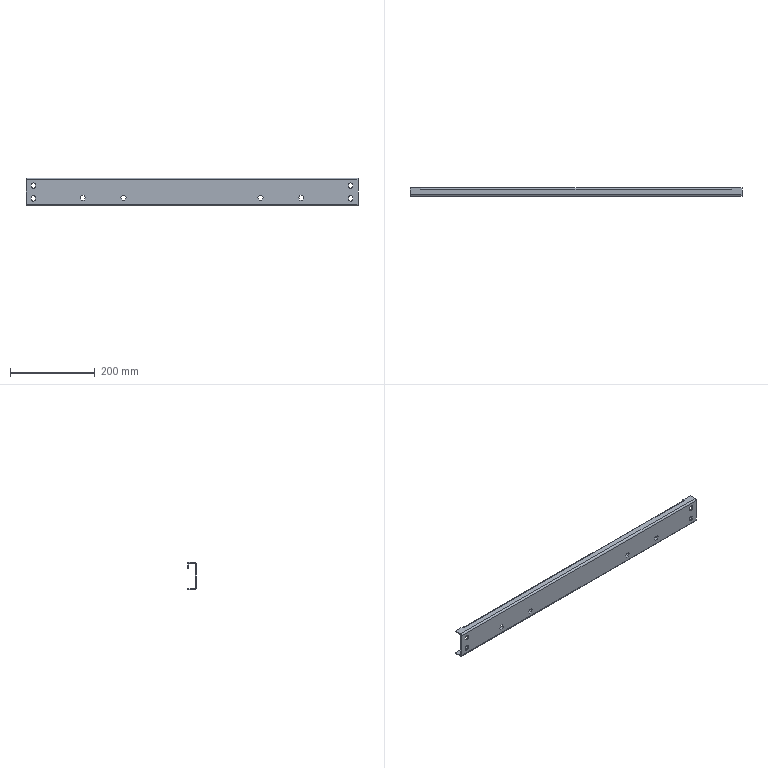Part | STEP file | Earthing switch reinforcing rib | 1 solid | 78 faces | box 785 x 20 x 65 mm | volume 208517 mm3 | plane 60 | cylinder 18 | commonest cylinder face diameters 9 x12 3 x3 8 x3